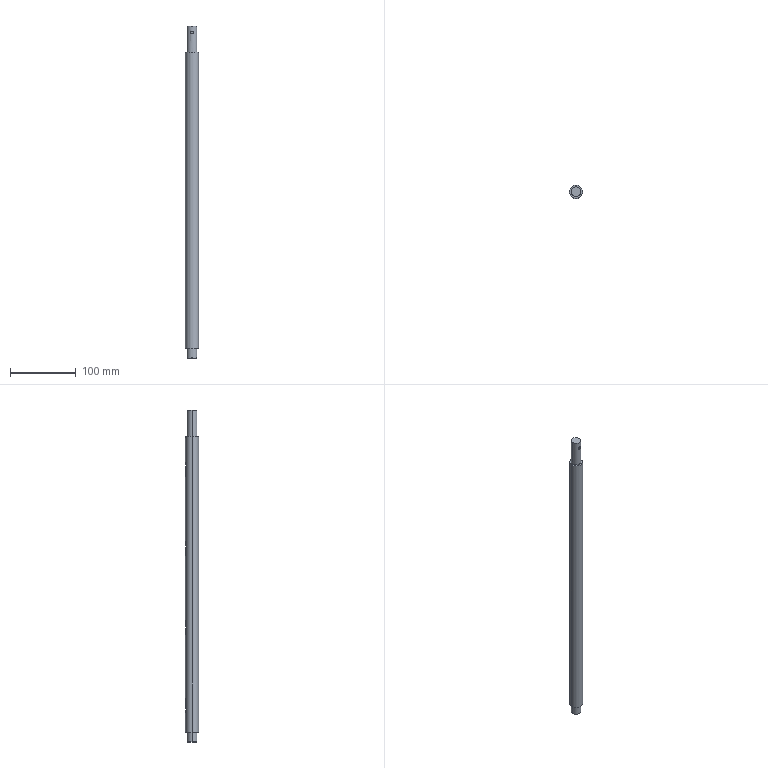Part | SolidWorks | features BaseBody 1 | 1 solid | 35 faces | box 20 x 20 x 505 mm | volume 149896 mm3 | plane 17 | cylinder 16 | cone 2 | commonest cylinder face diameters 6 x8 15 x4 4 x2 20 x2
STEP:
#1=CARTESIAN_POINT('',(2.,-6.,480.));
#2=VERTEX_POINT('',#1);
#3=CARTESIAN_POINT('',(-2.,-6.,480.));
#4=VERTEX_POINT('',#3);
#5=CARTESIAN_POINT('',(0.,-6.,480.));
#6=DIRECTION('',(0.,1.,0.));
#7=DIRECTION('',(1.,0.,0.));
#8=AXIS2_PLACEMENT_3D('',#5,#6,#7);
#9=CIRCLE('',#8,2.);
#10=EDGE_CURVE('',#2,#4,#9,.T.);
#11=ORIENTED_EDGE('',*,*,#10,.T.);
#12=CARTESIAN_POINT('',(-2.,-7.228,480.));
#13=VERTEX_POINT('',#12);
#14=CARTESIAN_POINT('',(-2.,-7.5,480.));
#15=DIRECTION('',(0.,-1.,0.));
#16=VECTOR('',#15,1000.);
#17=LINE('',#14,#16);
#18=EDGE_CURVE('',#4,#13,#17,.T.);
#19=ORIENTED_EDGE('',*,*,#18,.T.);
#20=CARTESIAN_POINT('',(2.,-7.228,480.));
#21=VERTEX_POINT('',#20);
#22=CARTESIAN_POINT('',(2.,-7.228,480.));
#23=CARTESIAN_POINT('',(2.,-7.228,479.867));
#24=CARTESIAN_POINT('',(1.987,-7.232,479.737));
#25=CARTESIAN_POINT('',(1.936,-7.246,479.481));
#26=CARTESIAN_POINT('',(1.897,-7.256,479.353));
#27=CARTESIAN_POINT('',(1.797,-7.282,479.112));
#28=CARTESIAN_POINT('',(1.735,-7.297,478.997));
#29=CARTESIAN_POINT('',(1.59,-7.33,478.78));
#30=CARTESIAN_POINT('',(1.506,-7.348,478.678));
#31=CARTESIAN_POINT('',(1.231,-7.401,478.403));
#32=CARTESIAN_POINT('',(1.009,-7.436,478.254));
#33=CARTESIAN_POINT('',(0.5289,-7.485,478.054));
#34=CARTESIAN_POINT('',(0.2655,-7.5,478.));
#35=CARTESIAN_POINT('',(-0.1326,-7.5,478.));
#36=CARTESIAN_POINT('',(-0.2629,-7.496,478.013));
#37=CARTESIAN_POINT('',(-0.5193,-7.483,478.064));
#38=CARTESIAN_POINT('',(-0.6466,-7.473,478.103));
#39=CARTESIAN_POINT('',(-0.8884,-7.448,478.203));
#40=CARTESIAN_POINT('',(-1.003,-7.433,478.265));
#41=CARTESIAN_POINT('',(-1.22,-7.401,478.41));
#42=CARTESIAN_POINT('',(-1.322,-7.383,478.494));
#43=CARTESIAN_POINT('',(-1.597,-7.33,478.769));
#44=CARTESIAN_POINT('',(-1.746,-7.295,478.991));
#45=CARTESIAN_POINT('',(-1.946,-7.244,479.471));
#46=CARTESIAN_POINT('',(-2.,-7.228,479.735));
#47=CARTESIAN_POINT('',(-2.,-7.228,480.));
#48=B_SPLINE_CURVE_WITH_KNOTS('',3,(#22,#23,#24,#25,#26,#27,#28,#29,#30,#31,#32,#33,#34,#35,#36,#37,#38,#39,#40,#41,#42,#43,#44,#45,#46,#47),.UNSPECIFIED.,.F.,.F.,(4,2,2,2,2,2,2,2,2,2,2,2,4),(0.009416,0.009808,0.0102,0.01059,0.01099,0.01177,0.01255,0.01295,0.01334,0.01373,0.01412,0.01491,0.01569),.UNSPECIFIED.);
#49=EDGE_CURVE('',#21,#13,#48,.T.);
#50=ORIENTED_EDGE('',*,*,#49,.F.);
#51=CARTESIAN_POINT('',(2.,-7.5,480.));
#52=DIRECTION('',(0.,-1.,0.));
#53=VECTOR('',#52,1000.);
#54=LINE('',#51,#53);
#55=EDGE_CURVE('',#2,#21,#54,.T.);
#56=ORIENTED_EDGE('',*,*,#55,.F.);
#57=EDGE_LOOP('',(#11,#19,#50,#56));
#58=FACE_OUTER_BOUND('',#57,.T.);
#59=CARTESIAN_POINT('',(0.,-7.5,480.));
#60=DIRECTION('',(0.,-1.,0.));
#61=DIRECTION('',(1.,0.,0.));
#62=AXIS2_PLACEMENT_3D('',#59,#60,#61);
#63=CYLINDRICAL_SURFACE('',#62,2.);
#64=ADVANCED_FACE('',(#58),#63,.F.);
#65=CARTESIAN_POINT('',(7.,0.,-15.));
#66=VERTEX_POINT('',#65);
#67=CARTESIAN_POINT('',(-7.,0.,-15.));
#68=VERTEX_POINT('',#67);
#69=CARTESIAN_POINT('',(0.,0.,-15.));
#70=DIRECTION('',(0.,0.,1.));
#71=DIRECTION('',(1.,0.,0.));
#72=AXIS2_PLACEMENT_3D('',#69,#70,#71);
#73=CIRCLE('',#72,7.);
#74=EDGE_CURVE('',#66,#68,#73,.T.);
#75=ORIENTED_EDGE('',*,*,#74,.T.);
#76=CARTESIAN_POINT('',(-7.5,0.,-14.5));
#77=VERTEX_POINT('',#76);
#78=CARTESIAN_POINT('',(-7.25,0.,-14.75));
#79=DIRECTION('',(-0.7071,0.,0.7071));
#80=VECTOR('',#79,1000.);
#81=LINE('',#78,#80);
#82=EDGE_CURVE('',#68,#77,#81,.T.);
#83=ORIENTED_EDGE('',*,*,#82,.T.);
#84=CARTESIAN_POINT('',(7.5,0.,-14.5));
#85=VERTEX_POINT('',#84);
#86=CARTESIAN_POINT('',(0.,0.,-14.5));
#87=DIRECTION('',(0.,0.,-1.));
#88=DIRECTION('',(1.,0.,0.));
#89=AXIS2_PLACEMENT_3D('',#86,#87,#88);
#90=CIRCLE('',#89,7.5);
#91=EDGE_CURVE('',#77,#85,#90,.T.);
#92=ORIENTED_EDGE('',*,*,#91,.T.);
#93=CARTESIAN_POINT('',(7.25,0.,-14.75));
#94=DIRECTION('',(0.7071,0.,0.7071));
#95=VECTOR('',#94,1000.);
#96=LINE('',#93,#95);
#97=EDGE_CURVE('',#66,#85,#96,.T.);
#98=ORIENTED_EDGE('',*,*,#97,.F.);
#99=EDGE_LOOP('',(#75,#83,#92,#98));
#100=FACE_OUTER_BOUND('',#99,.T.);
#101=CARTESIAN_POINT('',(0.,0.,-14.75));
#102=DIRECTION('',(0.,0.,1.));
#103=DIRECTION('',(1.,0.,0.));
#104=AXIS2_PLACEMENT_3D('',#101,#102,#103);
#105=CONICAL_SURFACE('',#104,7.25,0.7854);
#106=ADVANCED_FACE('',(#100),#105,.T.);
#107=ORIENTED_EDGE('',*,*,#91,.F.);
#108=CARTESIAN_POINT('',(-7.5,0.,0.));
#109=VERTEX_POINT('',#108);
#110=CARTESIAN_POINT('',(-7.5,0.,0.));
#111=DIRECTION('',(0.,0.,1.));
#112=VECTOR('',#111,1000.);
#113=LINE('',#110,#112);
#114=EDGE_CURVE('',#77,#109,#113,.T.);
#115=ORIENTED_EDGE('',*,*,#114,.T.);
#116=CARTESIAN_POINT('',(7.5,0.,0.));
#117=VERTEX_POINT('',#116);
#118=CARTESIAN_POINT('',(0.,0.,0.));
#119=DIRECTION('',(0.,0.,1.));
#120=DIRECTION('',(1.,0.,0.));
#121=AXIS2_PLACEMENT_3D('',#118,#119,#120);
#122=CIRCLE('',#121,7.5);
#123=EDGE_CURVE('',#117,#109,#122,.T.);
#124=ORIENTED_EDGE('',*,*,#123,.F.);
#125=CARTESIAN_POINT('',(7.5,0.,0.));
#126=DIRECTION('',(0.,0.,1.));
#127=VECTOR('',#126,1000.);
#128=LINE('',#125,#127);
#129=EDGE_CURVE('',#85,#117,#128,.T.);
#130=ORIENTED_EDGE('',*,*,#129,.F.);
#131=EDGE_LOOP('',(#107,#115,#124,#130));
#132=FACE_OUTER_BOUND('',#131,.T.);
#133=CARTESIAN_POINT('',(0.,0.,0.));
#134=DIRECTION('',(0.,0.,1.));
#135=DIRECTION('',(1.,0.,0.));
#136=AXIS2_PLACEMENT_3D('',#133,#134,#135);
#137=CYLINDRICAL_SURFACE('',#136,7.5);
#138=ADVANCED_FACE('',(#132),#137,.T.);
#139=CARTESIAN_POINT('',(7.5,0.,490.));
#140=VERTEX_POINT('',#139);
#141=CARTESIAN_POINT('',(-7.5,0.,490.));
#142=VERTEX_POINT('',#141);
#143=CARTESIAN_POINT('',(0.,0.,490.));
#144=DIRECTION('',(0.,0.,1.));
#145=DIRECTION('',(-1.,0.,0.));
#146=AXIS2_PLACEMENT_3D('',#143,#144,#145);
#147=CIRCLE('',#146,7.5);
#148=EDGE_CURVE('',#140,#142,#147,.T.);
#149=ORIENTED_EDGE('',*,*,#148,.F.);
#150=CARTESIAN_POINT('',(7.5,0.,450.));
#151=VERTEX_POINT('',#150);
#152=CARTESIAN_POINT('',(7.5,0.,450.));
#153=DIRECTION('',(0.,0.,-1.));
#154=VECTOR('',#153,1000.);
#155=LINE('',#152,#154);
#156=EDGE_CURVE('',#140,#151,#155,.T.);
#157=ORIENTED_EDGE('',*,*,#156,.T.);
#158=CARTESIAN_POINT('',(-7.5,0.,450.));
#159=VERTEX_POINT('',#158);
#160=CARTESIAN_POINT('',(0.,0.,450.));
#161=DIRECTION('',(0.,0.,-1.));
#162=DIRECTION('',(-1.,0.,0.));
#163=AXIS2_PLACEMENT_3D('',#160,#161,#162);
#164=CIRCLE('',#163,7.5);
#165=EDGE_CURVE('',#159,#151,#164,.T.);
#166=ORIENTED_EDGE('',*,*,#165,.F.);
#167=CARTESIAN_POINT('',(-7.5,0.,450.));
#168=DIRECTION('',(0.,0.,-1.));
#169=VECTOR('',#168,1000.);
#170=LINE('',#167,#169);
#171=EDGE_CURVE('',#142,#159,#170,.T.);
#172=ORIENTED_EDGE('',*,*,#171,.F.);
#173=EDGE_LOOP('',(#149,#157,#166,#172));
#174=FACE_OUTER_BOUND('',#173,.T.);
#175=CARTESIAN_POINT('',(0.,0.,450.));
#176=DIRECTION('',(0.,0.,-1.));
#177=DIRECTION('',(-1.,0.,0.));
#178=AXIS2_PLACEMENT_3D('',#175,#176,#177);
#179=CYLINDRICAL_SURFACE('',#178,7.5);
#180=ADVANCED_FACE('',(#174),#179,.T.);
#181=CARTESIAN_POINT('',(-3.,9.539,48.));
#182=VERTEX_POINT('',#181);
#183=CARTESIAN_POINT('',(-3.,9.539,32.));
#184=VERTEX_POINT('',#183);
#185=CARTESIAN_POINT('',(-3.,9.539,0.));
#186=DIRECTION('',(0.,0.,-1.));
#187=VECTOR('',#186,1000.);
#188=LINE('',#185,#187);
#189=EDGE_CURVE('',#182,#184,#188,.T.);
#190=ORIENTED_EDGE('',*,*,#189,.T.);
#191=CARTESIAN_POINT('',(3.,9.539,32.));
#192=VERTEX_POINT('',#191);
#193=CARTESIAN_POINT('',(-3.,9.539,32.));
#194=CARTESIAN_POINT('',(-3.,9.539,31.801));
#195=CARTESIAN_POINT('',(-2.98,9.546,31.605));
#196=CARTESIAN_POINT('',(-2.904,9.569,31.22));
#197=CARTESIAN_POINT('',(-2.845,9.587,31.029));
#198=CARTESIAN_POINT('',(-2.695,9.63,30.667));
#199=CARTESIAN_POINT('',(-2.602,9.656,30.495));
#200=CARTESIAN_POINT('',(-2.385,9.712,30.17));
#201=CARTESIAN_POINT('',(-2.259,9.742,30.017));
#202=CARTESIAN_POINT('',(-1.847,9.832,29.604));
#203=CARTESIAN_POINT('',(-1.515,9.891,29.381));
#204=CARTESIAN_POINT('',(-0.9743,9.954,29.156));
#205=CARTESIAN_POINT('',(-0.7844,9.971,29.098));
#206=CARTESIAN_POINT('',(-0.396,9.994,29.02));
#207=CARTESIAN_POINT('',(-0.1993,10.,29.));
#208=CARTESIAN_POINT('',(0.1994,10.,29.));
#209=CARTESIAN_POINT('',(0.3951,9.994,29.02));
#210=CARTESIAN_POINT('',(0.7799,9.971,29.097));
#211=CARTESIAN_POINT('',(0.971,9.954,29.155));
#212=CARTESIAN_POINT('',(1.334,9.912,29.306));
#213=CARTESIAN_POINT('',(1.505,9.887,29.398));
#214=CARTESIAN_POINT('',(1.831,9.832,29.615));
#215=CARTESIAN_POINT('',(1.984,9.802,29.741));
#216=CARTESIAN_POINT('',(2.396,9.713,30.153));
#217=CARTESIAN_POINT('',(2.619,9.652,30.486));
#218=CARTESIAN_POINT('',(2.844,9.587,31.026));
#219=CARTESIAN_POINT('',(2.902,9.57,31.216));
#220=CARTESIAN_POINT('',(2.98,9.546,31.604));
#221=CARTESIAN_POINT('',(3.,9.539,31.801));
#222=CARTESIAN_POINT('',(3.,9.539,32.));
#223=B_SPLINE_CURVE_WITH_KNOTS('',3,(#193,#194,#195,#196,#197,#198,#199,#200,#201,#202,#203,#204,#205,#206,#207,#208,#209,#210,#211,#212,#213,#214,#215,#216,#217,#218,#219,#220,#221,#222),.UNSPECIFIED.,.F.,.F.,(4,2,2,2,2,2,2,2,2,2,2,2,2,2,4),(0.,0.0005892,0.001178,0.001768,0.002357,0.003535,0.004125,0.004714,0.005303,0.005892,0.006482,0.007071,0.008249,0.008838,0.009428),.UNSPECIFIED.);
#224=EDGE_CURVE('',#184,#192,#223,.T.);
#225=ORIENTED_EDGE('',*,*,#224,.T.);
#226=CARTESIAN_POINT('',(3.,9.539,48.));
#227=VERTEX_POINT('',#226);
#228=CARTESIAN_POINT('',(3.,9.539,0.));
#229=DIRECTION('',(0.,0.,1.));
#230=VECTOR('',#229,1000.);
#231=LINE('',#228,#230);
#232=EDGE_CURVE('',#192,#227,#231,.T.);
#233=ORIENTED_EDGE('',*,*,#232,.T.);
#234=CARTESIAN_POINT('',(3.,9.539,48.));
#235=CARTESIAN_POINT('',(3.,9.539,48.199));
#236=CARTESIAN_POINT('',(2.98,9.546,48.395));
#237=CARTESIAN_POINT('',(2.904,9.569,48.78));
#238=CARTESIAN_POINT('',(2.845,9.587,48.971));
#239=CARTESIAN_POINT('',(2.695,9.63,49.333));
#240=CARTESIAN_POINT('',(2.602,9.656,49.505));
#241=CARTESIAN_POINT('',(2.385,9.712,49.83));
#242=CARTESIAN_POINT('',(2.259,9.742,49.983));
#243=CARTESIAN_POINT('',(1.847,9.832,50.396));
#244=CARTESIAN_POINT('',(1.515,9.891,50.619));
#245=CARTESIAN_POINT('',(0.9743,9.954,50.844));
#246=CARTESIAN_POINT('',(0.7844,9.971,50.902));
#247=CARTESIAN_POINT('',(0.396,9.994,50.98));
#248=CARTESIAN_POINT('',(0.1993,10.,51.));
#249=CARTESIAN_POINT('',(-0.1994,10.,51.));
#250=CARTESIAN_POINT('',(-0.3951,9.994,50.98));
#251=CARTESIAN_POINT('',(-0.7799,9.971,50.903));
#252=CARTESIAN_POINT('',(-0.971,9.954,50.845));
#253=CARTESIAN_POINT('',(-1.334,9.912,50.694));
#254=CARTESIAN_POINT('',(-1.505,9.887,50.602));
#255=CARTESIAN_POINT('',(-1.831,9.832,50.385));
#256=CARTESIAN_POINT('',(-1.984,9.802,50.259));
#257=CARTESIAN_POINT('',(-2.396,9.713,49.847));
#258=CARTESIAN_POINT('',(-2.619,9.652,49.514));
#259=CARTESIAN_POINT('',(-2.844,9.587,48.974));
#260=CARTESIAN_POINT('',(-2.902,9.57,48.784));
#261=CARTESIAN_POINT('',(-2.98,9.546,48.396));
#262=CARTESIAN_POINT('',(-3.,9.539,48.199));
#263=CARTESIAN_POINT('',(-3.,9.539,48.));
#264=B_SPLINE_CURVE_WITH_KNOTS('',3,(#234,#235,#236,#237,#238,#239,#240,#241,#242,#243,#244,#245,#246,#247,#248,#249,#250,#251,#252,#253,#254,#255,#256,#257,#258,#259,#260,#261,#262,#263),.UNSPECIFIED.,.F.,.F.,(4,2,2,2,2,2,2,2,2,2,2,2,2,2,4),(0.,0.0005892,0.001178,0.001768,0.002357,0.003535,0.004125,0.004714,0.005303,0.005892,0.006482,0.007071,0.008249,0.008838,0.009428),.UNSPECIFIED.);
#265=EDGE_CURVE('',#227,#182,#264,.T.);
#266=ORIENTED_EDGE('',*,*,#265,.T.);
#267=EDGE_LOOP('',(#190,#225,#233,#266));
#268=FACE_BOUND('',#267,.T.);
#269=CARTESIAN_POINT('',(-3.,9.539,168.));
#270=VERTEX_POINT('',#269);
#271=CARTESIAN_POINT('',(-3.,9.539,152.));
#272=VERTEX_POINT('',#271);
#273=CARTESIAN_POINT('',(-3.,9.539,0.));
#274=DIRECTION('',(0.,0.,-1.));
#275=VECTOR('',#274,1000.);
#276=LINE('',#273,#275);
#277=EDGE_CURVE('',#270,#272,#276,.T.);
#278=ORIENTED_EDGE('',*,*,#277,.T.);
#279=CARTESIAN_POINT('',(3.,9.539,152.));
#280=VERTEX_POINT('',#279);
#281=CARTESIAN_POINT('',(-3.,9.539,152.));
#282=CARTESIAN_POINT('',(-3.,9.539,151.801));
#283=CARTESIAN_POINT('',(-2.98,9.546,151.605));
#284=CARTESIAN_POINT('',(-2.904,9.569,151.22));
#285=CARTESIAN_POINT('',(-2.845,9.587,151.029));
#286=CARTESIAN_POINT('',(-2.695,9.63,150.667));
#287=CARTESIAN_POINT('',(-2.602,9.656,150.495));
#288=CARTESIAN_POINT('',(-2.385,9.712,150.17));
#289=CARTESIAN_POINT('',(-2.259,9.742,150.017));
#290=CARTESIAN_POINT('',(-1.847,9.832,149.604));
#291=CARTESIAN_POINT('',(-1.515,9.891,149.381));
#292=CARTESIAN_POINT('',(-0.9743,9.954,149.156));
#293=CARTESIAN_POINT('',(-0.7844,9.971,149.098));
#294=CARTESIAN_POINT('',(-0.396,9.994,149.02));
#295=CARTESIAN_POINT('',(-0.1993,10.,149.));
#296=CARTESIAN_POINT('',(0.1994,10.,149.));
#297=CARTESIAN_POINT('',(0.3951,9.994,149.02));
#298=CARTESIAN_POINT('',(0.7799,9.971,149.097));
#299=CARTESIAN_POINT('',(0.971,9.954,149.155));
#300=CARTESIAN_POINT('',(1.334,9.912,149.306));
#301=CARTESIAN_POINT('',(1.505,9.887,149.398));
#302=CARTESIAN_POINT('',(1.831,9.832,149.615));
#303=CARTESIAN_POINT('',(1.984,9.802,149.741));
#304=CARTESIAN_POINT('',(2.396,9.713,150.153));
#305=CARTESIAN_POINT('',(2.619,9.652,150.486));
#306=CARTESIAN_POINT('',(2.844,9.587,151.026));
#307=CARTESIAN_POINT('',(2.902,9.57,151.216));
#308=CARTESIAN_POINT('',(2.98,9.546,151.604));
#309=CARTESIAN_POINT('',(3.,9.539,151.801));
#310=CARTESIAN_POINT('',(3.,9.539,152.));
#311=B_SPLINE_CURVE_WITH_KNOTS('',3,(#281,#282,#283,#284,#285,#286,#287,#288,#289,#290,#291,#292,#293,#294,#295,#296,#297,#298,#299,#300,#301,#302,#303,#304,#305,#306,#307,#308,#309,#310),.UNSPECIFIED.,.F.,.F.,(4,2,2,2,2,2,2,2,2,2,2,2,2,2,4),(0.,0.0005892,0.001178,0.001768,0.002357,0.003535,0.004125,0.004714,0.005303,0.005892,0.006482,0.007071,0.008249,0.008838,0.009428),.UNSPECIFIED.);
#312=EDGE_CURVE('',#272,#280,#311,.T.);
#313=ORIENTED_EDGE('',*,*,#312,.T.);
#314=CARTESIAN_POINT('',(3.,9.539,168.));
#315=VERTEX_POINT('',#314);
#316=CARTESIAN_POINT('',(3.,9.539,0.));
#317=DIRECTION('',(0.,0.,1.));
#318=VECTOR('',#317,1000.);
#319=LINE('',#316,#318);
#320=EDGE_CURVE('',#280,#315,#319,.T.);
#321=ORIENTED_EDGE('',*,*,#320,.T.);
#322=CARTESIAN_POINT('',(3.,9.539,168.));
#323=CARTESIAN_POINT('',(3.,9.539,168.199));
#324=CARTESIAN_POINT('',(2.98,9.546,168.395));
#325=CARTESIAN_POINT('',(2.904,9.569,168.78));
#326=CARTESIAN_POINT('',(2.845,9.587,168.971));
#327=CARTESIAN_POINT('',(2.695,9.63,169.333));
#328=CARTESIAN_POINT('',(2.602,9.656,169.505));
#329=CARTESIAN_POINT('',(2.385,9.712,169.83));
#330=CARTESIAN_POINT('',(2.259,9.742,169.983));
#331=CARTESIAN_POINT('',(1.847,9.832,170.396));
#332=CARTESIAN_POINT('',(1.515,9.891,170.619));
#333=CARTESIAN_POINT('',(0.9743,9.954,170.844));
#334=CARTESIAN_POINT('',(0.7844,9.971,170.902));
#335=CARTESIAN_POINT('',(0.396,9.994,170.98));
#336=CARTESIAN_POINT('',(0.1993,10.,171.));
#337=CARTESIAN_POINT('',(-0.1994,10.,171.));
#338=CARTESIAN_POINT('',(-0.3951,9.994,170.98));
#339=CARTESIAN_POINT('',(-0.7799,9.971,170.903));
#340=CARTESIAN_POINT('',(-0.971,9.954,170.845));
#341=CARTESIAN_POINT('',(-1.334,9.912,170.694));
#342=CARTESIAN_POINT('',(-1.505,9.887,170.602));
#343=CARTESIAN_POINT('',(-1.831,9.832,170.385));
#344=CARTESIAN_POINT('',(-1.984,9.802,170.259));
#345=CARTESIAN_POINT('',(-2.396,9.713,169.847));
#346=CARTESIAN_POINT('',(-2.619,9.652,169.514));
#347=CARTESIAN_POINT('',(-2.844,9.587,168.974));
#348=CARTESIAN_POINT('',(-2.902,9.57,168.784));
#349=CARTESIAN_POINT('',(-2.98,9.546,168.396));
#350=CARTESIAN_POINT('',(-3.,9.539,168.199));
#351=CARTESIAN_POINT('',(-3.,9.539,168.));
#352=B_SPLINE_CURVE_WITH_KNOTS('',3,(#322,#323,#324,#325,#326,#327,#328,#329,#330,#331,#332,#333,#334,#335,#336,#337,#338,#339,#340,#341,#342,#343,#344,#345,#346,#347,#348,#349,#350,#351),.UNSPECIFIED.,.F.,.F.,(4,2,2,2,2,2,2,2,2,2,2,2,2,2,4),(0.,0.0005892,0.001178,0.001768,0.002357,0.003535,0.004125,0.004714,0.005303,0.005892,0.006482,0.007071,0.008249,0.008838,0.009428),.UNSPECIFIED.);
#353=EDGE_CURVE('',#315,#270,#352,.T.);
#354=ORIENTED_EDGE('',*,*,#353,.T.);
#355=EDGE_LOOP('',(#278,#313,#321,#354));
#356=FACE_BOUND('',#355,.T.);
#357=CARTESIAN_POINT('',(-3.,9.539,288.));
#358=VERTEX_POINT('',#357);
#359=CARTESIAN_POINT('',(-3.,9.539,272.));
#360=VERTEX_POINT('',#359);
#361=CARTESIAN_POINT('',(-3.,9.539,0.));
#362=DIRECTION('',(0.,0.,-1.));
#363=VECTOR('',#362,1000.);
#364=LINE('',#361,#363);
#365=EDGE_CURVE('',#358,#360,#364,.T.);
#366=ORIENTED_EDGE('',*,*,#365,.T.);
#367=CARTESIAN_POINT('',(3.,9.539,272.));
#368=VERTEX_POINT('',#367);
#369=CARTESIAN_POINT('',(-3.,9.539,272.));
#370=CARTESIAN_POINT('',(-3.,9.539,271.801));
#371=CARTESIAN_POINT('',(-2.98,9.546,271.605));
#372=CARTESIAN_POINT('',(-2.904,9.569,271.22));
#373=CARTESIAN_POINT('',(-2.845,9.587,271.029));
#374=CARTESIAN_POINT('',(-2.695,9.63,270.667));
#375=CARTESIAN_POINT('',(-2.602,9.656,270.495));
#376=CARTESIAN_POINT('',(-2.385,9.712,270.17));
#377=CARTESIAN_POINT('',(-2.259,9.742,270.017));
#378=CARTESIAN_POINT('',(-1.847,9.832,269.604));
#379=CARTESIAN_POINT('',(-1.515,9.891,269.381));
#380=CARTESIAN_POINT('',(-0.9743,9.954,269.156));
#381=CARTESIAN_POINT('',(-0.7844,9.971,269.098));
#382=CARTESIAN_POINT('',(-0.396,9.994,269.02));
#383=CARTESIAN_POINT('',(-0.1993,10.,269.));
#384=CARTESIAN_POINT('',(0.1994,10.,269.));
#385=CARTESIAN_POINT('',(0.3951,9.994,269.02));
#386=CARTESIAN_POINT('',(0.7799,9.971,269.097));
#387=CARTESIAN_POINT('',(0.971,9.954,269.155));
#388=CARTESIAN_POINT('',(1.334,9.912,269.306));
#389=CARTESIAN_POINT('',(1.505,9.887,269.398));
#390=CARTESIAN_POINT('',(1.831,9.832,269.615));
#391=CARTESIAN_POINT('',(1.984,9.802,269.741));
#392=CARTESIAN_POINT('',(2.396,9.713,270.153));
#393=CARTESIAN_POINT('',(2.619,9.652,270.486));
#394=CARTESIAN_POINT('',(2.844,9.587,271.026));
#395=CARTESIAN_POINT('',(2.902,9.57,271.216));
#396=CARTESIAN_POINT('',(2.98,9.546,271.604));
#397=CARTESIAN_POINT('',(3.,9.539,271.801));
#398=CARTESIAN_POINT('',(3.,9.539,272.));
#399=B_SPLINE_CURVE_WITH_KNOTS('',3,(#369,#370,#371,#372,#373,#374,#375,#376,#377,#378,#379,#380,#381,#382,#383,#384,#385,#386,#387,#388,#389,#390,#391,#392,#393,#394,#395,#396,#397,#398),.UNSPECIFIED.,.F.,.F.,(4,2,2,2,2,2,2,2,2,2,2,2,2,2,4),(0.,0.0005892,0.001178,0.001768,0.002357,0.003535,0.004125,0.004714,0.005303,0.005892,0.006482,0.007071,0.008249,0.008838,0.009428),.UNSPECIFIED.);
#400=EDGE_CURVE('',#360,#368,#399,.T.);
#401=ORIENTED_EDGE('',*,*,#400,.T.);
#402=CARTESIAN_POINT('',(3.,9.539,288.));
#403=VERTEX_POINT('',#402);
#404=CARTESIAN_POINT('',(3.,9.539,0.));
#405=DIRECTION('',(0.,0.,1.));
#406=VECTOR('',#405,1000.);
#407=LINE('',#404,#406);
#408=EDGE_CURVE('',#368,#403,#407,.T.);
#409=ORIENTED_EDGE('',*,*,#408,.T.);
#410=CARTESIAN_POINT('',(3.,9.539,288.));
#411=CARTESIAN_POINT('',(3.,9.539,288.199));
#412=CARTESIAN_POINT('',(2.98,9.546,288.395));
#413=CARTESIAN_POINT('',(2.904,9.569,288.78));
#414=CARTESIAN_POINT('',(2.845,9.587,288.971));
#415=CARTESIAN_POINT('',(2.695,9.63,289.333));
#416=CARTESIAN_POINT('',(2.602,9.656,289.505));
#417=CARTESIAN_POINT('',(2.385,9.712,289.83));
#418=CARTESIAN_POINT('',(2.259,9.742,289.983));
#419=CARTESIAN_POINT('',(1.847,9.832,290.396));
#420=CARTESIAN_POINT('',(1.515,9.891,290.619));
#421=CARTESIAN_POINT('',(0.9743,9.954,290.844));
#422=CARTESIAN_POINT('',(0.7844,9.971,290.902));
#423=CARTESIAN_POINT('',(0.396,9.994,290.98));
#424=CARTESIAN_POINT('',(0.1993,10.,291.));
#425=CARTESIAN_POINT('',(-0.1994,10.,291.));
#426=CARTESIAN_POINT('',(-0.3951,9.994,290.98));
#427=CARTESIAN_POINT('',(-0.7799,9.971,290.903));
#428=CARTESIAN_POINT('',(-0.971,9.954,290.845));
#429=CARTESIAN_POINT('',(-1.334,9.912,290.694));
#430=CARTESIAN_POINT('',(-1.505,9.887,290.602));
#431=CARTESIAN_POINT('',(-1.831,9.832,290.385));
#432=CARTESIAN_POINT('',(-1.984,9.802,290.259));
#433=CARTESIAN_POINT('',(-2.396,9.713,289.847));
#434=CARTESIAN_POINT('',(-2.619,9.652,289.514));
#435=CARTESIAN_POINT('',(-2.844,9.587,288.974));
#436=CARTESIAN_POINT('',(-2.902,9.57,288.784));
#437=CARTESIAN_POINT('',(-2.98,9.546,288.396));
#438=CARTESIAN_POINT('',(-3.,9.539,288.199));
#439=CARTESIAN_POINT('',(-3.,9.539,288.));
#440=B_SPLINE_CURVE_WITH_KNOTS('',3,(#410,#411,#412,#413,#414,#415,#416,#417,#418,#419,#420,#421,#422,#423,#424,#425,#426,#427,#428,#429,#430,#431,#432,#433,#434,#435,#436,#437,#438,#439),.UNSPECIFIED.,.F.,.F.,(4,2,2,2,2,2,2,2,2,2,2,2,2,2,4),(0.,0.0005892,0.001178,0.001768,0.002357,0.003535,0.004125,0.004714,0.005303,0.005892,0.006482,0.007071,0.008249,0.008838,0.009428),.UNSPECIFIED.);
#441=EDGE_CURVE('',#403,#358,#440,.T.);
#442=ORIENTED_EDGE('',*,*,#441,.T.);
#443=EDGE_LOOP('',(#366,#401,#409,#442));
#444=FACE_BOUND('',#443,.T.);
#445=CARTESIAN_POINT('',(-3.,9.539,408.));
#446=VERTEX_POINT('',#445);
#447=CARTESIAN_POINT('',(-3.,9.539,392.));
#448=VERTEX_POINT('',#447);
#449=CARTESIAN_POINT('',(-3.,9.539,0.));
#450=DIRECTION('',(0.,0.,-1.));
#451=VECTOR('',#450,1000.);
#452=LINE('',#449,#451);
#453=EDGE_CURVE('',#446,#448,#452,.T.);
#454=ORIENTED_EDGE('',*,*,#453,.T.);
#455=CARTESIAN_POINT('',(3.,9.539,392.));
#456=VERTEX_POINT('',#455);
#457=CARTESIAN_POINT('',(-3.,9.539,392.));
#458=CARTESIAN_POINT('',(-3.,9.539,391.801));
#459=CARTESIAN_POINT('',(-2.98,9.546,391.605));
#460=CARTESIAN_POINT('',(-2.904,9.569,391.22));
#461=CARTESIAN_POINT('',(-2.845,9.587,391.029));
#462=CARTESIAN_POINT('',(-2.695,9.63,390.667));
#463=CARTESIAN_POINT('',(-2.602,9.656,390.495));
#464=CARTESIAN_POINT('',(-2.385,9.712,390.17));
#465=CARTESIAN_POINT('',(-2.259,9.742,390.017));
#466=CARTESIAN_POINT('',(-1.847,9.832,389.604));
#467=CARTESIAN_POINT('',(-1.515,9.891,389.381));
#468=CARTESIAN_POINT('',(-0.9743,9.954,389.156));
#469=CARTESIAN_POINT('',(-0.7844,9.971,389.098));
#470=CARTESIAN_POINT('',(-0.396,9.994,389.02));
#471=CARTESIAN_POINT('',(-0.1993,10.,389.));
#472=CARTESIAN_POINT('',(0.1994,10.,389.));
#473=CARTESIAN_POINT('',(0.3951,9.994,389.02));
#474=CARTESIAN_POINT('',(0.7799,9.971,389.097));
#475=CARTESIAN_POINT('',(0.971,9.954,389.155));
#476=CARTESIAN_POINT('',(1.334,9.912,389.306));
#477=CARTESIAN_POINT('',(1.505,9.887,389.398));
#478=CARTESIAN_POINT('',(1.831,9.832,389.615));
#479=CARTESIAN_POINT('',(1.984,9.802,389.741));
#480=CARTESIAN_POINT('',(2.396,9.713,390.153));
#481=CARTESIAN_POINT('',(2.619,9.652,390.486));
#482=CARTESIAN_POINT('',(2.844,9.587,391.026));
#483=CARTESIAN_POINT('',(2.902,9.57,391.216));
#484=CARTESIAN_POINT('',(2.98,9.546,391.604));
#485=CARTESIAN_POINT('',(3.,9.539,391.801));
#486=CARTESIAN_POINT('',(3.,9.539,392.));
#487=B_SPLINE_CURVE_WITH_KNOTS('',3,(#457,#458,#459,#460,#461,#462,#463,#464,#465,#466,#467,#468,#469,#470,#471,#472,#473,#474,#475,#476,#477,#478,#479,#480,#481,#482,#483,#484,#485,#486),.UNSPECIFIED.,.F.,.F.,(4,2,2,2,2,2,2,2,2,2,2,2,2,2,4),(0.,0.0005892,0.001178,0.001768,0.002357,0.003535,0.004125,0.004714,0.005303,0.005892,0.006482,0.007071,0.008249,0.008838,0.009428),.UNSPECIFIED.);
#488=EDGE_CURVE('',#448,#456,#487,.T.);
#489=ORIENTED_EDGE('',*,*,#488,.T.);
#490=CARTESIAN_POINT('',(3.,9.539,408.));
#491=VERTEX_POINT('',#490);
#492=CARTESIAN_POINT('',(3.,9.539,0.));
#493=DIRECTION('',(0.,0.,1.));
#494=VECTOR('',#493,1000.);
#495=LINE('',#492,#494);
#496=EDGE_CURVE('',#456,#491,#495,.T.);
#497=ORIENTED_EDGE('',*,*,#496,.T.);
#498=CARTESIAN_POINT('',(3.,9.539,408.));
#499=CARTESIAN_POINT('',(3.,9.539,408.199));
#500=CARTESIAN_POINT('',(2.98,9.546,408.395));
#501=CARTESIAN_POINT('',(2.904,9.569,408.78));
#502=CARTESIAN_POINT('',(2.845,9.587,408.971));
#503=CARTESIAN_POINT('',(2.695,9.63,409.333));
#504=CARTESIAN_POINT('',(2.602,9.656,409.505));
#505=CARTESIAN_POINT('',(2.385,9.712,409.83));
#506=CARTESIAN_POINT('',(2.259,9.742,409.983));
#507=CARTESIAN_POINT('',(1.847,9.832,410.396));
#508=CARTESIAN_POINT('',(1.515,9.891,410.619));
#509=CARTESIAN_POINT('',(0.9743,9.954,410.844));
#510=CARTESIAN_POINT('',(0.7844,9.971,410.902));
#511=CARTESIAN_POINT('',(0.396,9.994,410.98));
#512=CARTESIAN_POINT('',(0.1993,10.,411.));
#513=CARTESIAN_POINT('',(-0.1994,10.,411.));
#514=CARTESIAN_POINT('',(-0.3951,9.994,410.98));
#515=CARTESIAN_POINT('',(-0.7799,9.971,410.903));
#516=CARTESIAN_POINT('',(-0.971,9.954,410.845));
#517=CARTESIAN_POINT('',(-1.334,9.912,410.694));
#518=CARTESIAN_POINT('',(-1.505,9.887,410.602));
#519=CARTESIAN_POINT('',(-1.831,9.832,410.385));
#520=CARTESIAN_POINT('',(-1.984,9.802,410.259));
#521=CARTESIAN_POINT('',(-2.396,9.713,409.847));
#522=CARTESIAN_POINT('',(-2.619,9.652,409.514));
#523=CARTESIAN_POINT('',(-2.844,9.587,408.974));
#524=CARTESIAN_POINT('',(-2.902,9.57,408.784));
#525=CARTESIAN_POINT('',(-2.98,9.546,408.396));
#526=CARTESIAN_POINT('',(-3.,9.539,408.199));
#527=CARTESIAN_POINT('',(-3.,9.539,408.));
#528=B_SPLINE_CURVE_WITH_KNOTS('',3,(#498,#499,#500,#501,#502,#503,#504,#505,#506,#507,#508,#509,#510,#511,#512,#513,#514,#515,#516,#517,#518,#519,#520,#521,#522,#523,#524,#525,#526,#527),.UNSPECIFIED.,.F.,.F.,(4,2,2,2,2,2,2,2,2,2,2,2,2,2,4),(0.,0.0005892,0.001178,0.001768,0.002357,0.003535,0.004125,0.004714,0.005303,0.005892,0.006482,0.007071,0.008249,0.008838,0.009428),.UNSPECIFIED.);
#529=EDGE_CURVE('',#491,#446,#528,.T.);
#530=ORIENTED_EDGE('',*,*,#529,.T.);
#531=EDGE_LOOP('',(#454,#489,#497,#530));
#532=FACE_BOUND('',#531,.T.);
#533=CARTESIAN_POINT('',(10.,0.,450.));
#534=VERTEX_POINT('',#533);
#535=CARTESIAN_POINT('',(-10.,0.,450.));
#536=VERTEX_POINT('',#535);
#537=CARTESIAN_POINT('',(0.,0.,450.));
#538=DIRECTION('',(0.,0.,1.));
#539=DIRECTION('',(-1.,0.,0.));
#540=AXIS2_PLACEMENT_3D('',#537,#538,#539);
#541=CIRCLE('',#540,10.);
#542=EDGE_CURVE('',#534,#536,#541,.T.);
#543=ORIENTED_EDGE('',*,*,#542,.F.);
#544=CARTESIAN_POINT('',(10.,0.,0.));
#545=VERTEX_POINT('',#544);
#546=CARTESIAN_POINT('',(10.,0.,0.));
#547=DIRECTION('',(0.,0.,-1.));
#548=VECTOR('',#547,1000.);
#549=LINE('',#546,#548);
#550=EDGE_CURVE('',#534,#545,#549,.T.);
#551=ORIENTED_EDGE('',*,*,#550,.T.);
#552=CARTESIAN_POINT('',(-10.,0.,0.));
#553=VERTEX_POINT('',#552);
#554=CARTESIAN_POINT('',(0.,0.,0.));
#555=DIRECTION('',(0.,0.,-1.));
#556=DIRECTION('',(-1.,0.,0.));
#557=AXIS2_PLACEMENT_3D('',#554,#555,#556);
#558=CIRCLE('',#557,10.);
#559=EDGE_CURVE('',#553,#545,#558,.T.);
#560=ORIENTED_EDGE('',*,*,#559,.F.);
#561=CARTESIAN_POINT('',(-10.,0.,0.));
#562=DIRECTION('',(0.,0.,-1.));
#563=VECTOR('',#562,1000.);
#564=LINE('',#561,#563);
#565=EDGE_CURVE('',#536,#553,#564,.T.);
#566=ORIENTED_EDGE('',*,*,#565,.F.);
#567=EDGE_LOOP('',(#543,#551,#560,#566));
#568=FACE_OUTER_BOUND('',#567,.T.);
#569=CARTESIAN_POINT('',(0.,0.,0.));
#570=DIRECTION('',(0.,0.,-1.));
#571=DIRECTION('',(-1.,0.,0.));
#572=AXIS2_PLACEMENT_3D('',#569,#570,#571);
#573=CYLINDRICAL_SURFACE('',#572,10.);
#574=ADVANCED_FACE('',(#268,#356,#444,#532,#568),#573,.T.);
#575=ORIENTED_EDGE('',*,*,#10,.F.);
#576=CARTESIAN_POINT('',(0.,-6.,480.));
#577=DIRECTION('',(0.,1.,0.));
#578=DIRECTION('',(1.,0.,0.));
#579=AXIS2_PLACEMENT_3D('',#576,#577,#578);
#580=CIRCLE('',#579,2.);
#581=EDGE_CURVE('',#4,#2,#580,.T.);
#582=ORIENTED_EDGE('',*,*,#581,.F.);
#583=EDGE_LOOP('',(#575,#582));
#584=FACE_OUTER_BOUND('',#583,.T.);
#585=CARTESIAN_POINT('',(0.,-6.,480.));
#586=DIRECTION('',(0.,1.,0.));
#587=DIRECTION('',(1.,0.,0.));
#588=AXIS2_PLACEMENT_3D('',#585,#586,#587);
#589=PLANE('',#588);
#590=ADVANCED_FACE('',(#584),#589,.F.);
#591=ORIENTED_EDGE('',*,*,#232,.F.);
#592=CARTESIAN_POINT('',(3.,7.5,32.));
#593=VERTEX_POINT('',#592);
#594=CARTESIAN_POINT('',(3.,10.,32.));
#595=DIRECTION('',(0.,-1.,0.));
#596=VECTOR('',#595,1000.);
#597=LINE('',#594,#596);
#598=EDGE_CURVE('',#192,#593,#597,.T.);
#599=ORIENTED_EDGE('',*,*,#598,.T.);
#600=CARTESIAN_POINT('',(3.,7.5,48.));
#601=VERTEX_POINT('',#600);
#602=CARTESIAN_POINT('',(3.,7.5,48.));
#603=DIRECTION('',(0.,0.,1.));
#604=VECTOR('',#603,1000.);
#605=LINE('',#602,#604);
#606=EDGE_CURVE('',#593,#601,#605,.T.);
#607=ORIENTED_EDGE('',*,*,#606,.T.);
#608=CARTESIAN_POINT('',(3.,10.,48.));
#609=DIRECTION('',(0.,-1.,0.));
#610=VECTOR('',#609,1000.);
#611=LINE('',#608,#610);
#612=EDGE_CURVE('',#227,#601,#611,.T.);
#613=ORIENTED_EDGE('',*,*,#612,.F.);
#614=EDGE_LOOP('',(#591,#599,#607,#613));
#615=FACE_OUTER_BOUND('',#614,.T.);
#616=CARTESIAN_POINT('',(3.,10.,32.));
#617=DIRECTION('',(1.,0.,0.));
#618=DIRECTION('',(0.,0.,1.));
#619=AXIS2_PLACEMENT_3D('',#616,#617,#618);
#620=PLANE('',#619);
#621=ADVANCED_FACE('',(#615),#620,.F.);
#622=ORIENTED_EDGE('',*,*,#265,.F.);
#623=ORIENTED_EDGE('',*,*,#612,.T.);
#624=CARTESIAN_POINT('',(-3.,7.5,48.));
#625=VERTEX_POINT('',#624);
#626=CARTESIAN_POINT('',(0.,7.5,48.));
#627=DIRECTION('',(0.,-1.,0.));
#628=DIRECTION('',(-1.,0.,0.));
#629=AXIS2_PLACEMENT_3D('',#626,#627,#628);
#630=CIRCLE('',#629,3.);
#631=EDGE_CURVE('',#601,#625,#630,.T.);
#632=ORIENTED_EDGE('',*,*,#631,.T.);
#633=CARTESIAN_POINT('',(-3.,10.,48.));
#634=DIRECTION('',(0.,-1.,0.));
#635=VECTOR('',#634,1000.);
#636=LINE('',#633,#635);
#637=EDGE_CURVE('',#182,#625,#636,.T.);
#638=ORIENTED_EDGE('',*,*,#637,.F.);
#639=EDGE_LOOP('',(#622,#623,#632,#638));
#640=FACE_OUTER_BOUND('',#639,.T.);
#641=CARTESIAN_POINT('',(0.,10.,48.));
#642=DIRECTION('',(0.,1.,0.));
#643=DIRECTION('',(-1.,0.,0.));
#644=AXIS2_PLACEMENT_3D('',#641,#642,#643);
#645=CYLINDRICAL_SURFACE('',#644,3.);
#646=ADVANCED_FACE('',(#640),#645,.F.);
#647=ORIENTED_EDGE('',*,*,#189,.F.);
#648=ORIENTED_EDGE('',*,*,#637,.T.);
#649=CARTESIAN_POINT('',(-3.,7.5,32.));
#650=VERTEX_POINT('',#649);
#651=CARTESIAN_POINT('',(-3.,7.5,32.));
#652=DIRECTION('',(0.,0.,-1.));
#653=VECTOR('',#652,1000.);
#654=LINE('',#651,#653);
#655=EDGE_CURVE('',#625,#650,#654,.T.);
#656=ORIENTED_EDGE('',*,*,#655,.T.);
#657=CARTESIAN_POINT('',(-3.,10.,32.));
#658=DIRECTION('',(0.,-1.,0.));
#659=VECTOR('',#658,1000.);
#660=LINE('',#657,#659);
#661=EDGE_CURVE('',#184,#650,#660,.T.);
#662=ORIENTED_EDGE('',*,*,#661,.F.);
#663=EDGE_LOOP('',(#647,#648,#656,#662));
#664=FACE_OUTER_BOUND('',#663,.T.);
#665=CARTESIAN_POINT('',(-3.,10.,48.));
#666=DIRECTION('',(-1.,0.,0.));
#667=DIRECTION('',(0.,0.,1.));
#668=AXIS2_PLACEMENT_3D('',#665,#666,#667);
#669=PLANE('',#668);
#670=ADVANCED_FACE('',(#664),#669,.F.);
#671=ORIENTED_EDGE('',*,*,#598,.F.);
#672=ORIENTED_EDGE('',*,*,#224,.F.);
#673=ORIENTED_EDGE('',*,*,#661,.T.);
#674=CARTESIAN_POINT('',(0.,7.5,32.));
#675=DIRECTION('',(0.,-1.,0.));
#676=DIRECTION('',(1.,0.,0.));
#677=AXIS2_PLACEMENT_3D('',#674,#675,#676);
#678=CIRCLE('',#677,3.);
#679=EDGE_CURVE('',#650,#593,#678,.T.);
#680=ORIENTED_EDGE('',*,*,#679,.T.);
#681=EDGE_LOOP('',(#671,#672,#673,#680));
#682=FACE_OUTER_BOUND('',#681,.T.);
#683=CARTESIAN_POINT('',(0.,10.,32.));
#684=DIRECTION('',(0.,1.,0.));
#685=DIRECTION('',(1.,0.,0.));
#686=AXIS2_PLACEMENT_3D('',#683,#684,#685);
#687=CYLINDRICAL_SURFACE('',#686,3.);
#688=ADVANCED_FACE('',(#682),#687,.F.);
#689=ORIENTED_EDGE('',*,*,#679,.F.);
#690=ORIENTED_EDGE('',*,*,#655,.F.);
#691=ORIENTED_EDGE('',*,*,#631,.F.);
#692=ORIENTED_EDGE('',*,*,#606,.F.);
#693=EDGE_LOOP('',(#689,#690,#691,#692));
#694=FACE_OUTER_BOUND('',#693,.T.);
#695=CARTESIAN_POINT('',(0.,7.5,30.967));
#696=DIRECTION('',(0.,1.,0.));
#697=DIRECTION('',(1.,0.,0.));
#698=AXIS2_PLACEMENT_3D('',#695,#696,#697);
#699=PLANE('',#698);
#700=ADVANCED_FACE('',(#694),#699,.T.);
#701=ORIENTED_EDGE('',*,*,#320,.F.);
#702=CARTESIAN_POINT('',(3.,7.5,152.));
#703=VERTEX_POINT('',#702);
#704=CARTESIAN_POINT('',(3.,10.,152.));
#705=DIRECTION('',(0.,-1.,0.));
#706=VECTOR('',#705,1000.);
#707=LINE('',#704,#706);
#708=EDGE_CURVE('',#280,#703,#707,.T.);
#709=ORIENTED_EDGE('',*,*,#708,.T.);
#710=CARTESIAN_POINT('',(3.,7.5,168.));
#711=VERTEX_POINT('',#710);
#712=CARTESIAN_POINT('',(3.,7.5,168.));
#713=DIRECTION('',(0.,0.,1.));
#714=VECTOR('',#713,1000.);
#715=LINE('',#712,#714);
#716=EDGE_CURVE('',#703,#711,#715,.T.);
#717=ORIENTED_EDGE('',*,*,#716,.T.);
#718=CARTESIAN_POINT('',(3.,10.,168.));
#719=DIRECTION('',(0.,-1.,0.));
#720=VECTOR('',#719,1000.);
#721=LINE('',#718,#720);
#722=EDGE_CURVE('',#315,#711,#721,.T.);
#723=ORIENTED_EDGE('',*,*,#722,.F.);
#724=EDGE_LOOP('',(#701,#709,#717,#723));
#725=FACE_OUTER_BOUND('',#724,.T.);
#726=CARTESIAN_POINT('',(3.,10.,152.));
#727=DIRECTION('',(1.,0.,0.));
#728=DIRECTION('',(0.,0.,1.));
#729=AXIS2_PLACEMENT_3D('',#726,#727,#728);
#730=PLANE('',#729);
#731=ADVANCED_FACE('',(#725),#730,.F.);
#732=ORIENTED_EDGE('',*,*,#353,.F.);
#733=ORIENTED_EDGE('',*,*,#722,.T.);
#734=CARTESIAN_POINT('',(-3.,7.5,168.));
#735=VERTEX_POINT('',#734);
#736=CARTESIAN_POINT('',(0.,7.5,168.));
#737=DIRECTION('',(0.,-1.,0.));
#738=DIRECTION('',(-1.,0.,0.));
#739=AXIS2_PLACEMENT_3D('',#736,#737,#738);
#740=CIRCLE('',#739,3.);
#741=EDGE_CURVE('',#711,#735,#740,.T.);
#742=ORIENTED_EDGE('',*,*,#741,.T.);
#743=CARTESIAN_POINT('',(-3.,10.,168.));
#744=DIRECTION('',(0.,-1.,0.));
#745=VECTOR('',#744,1000.);
#746=LINE('',#743,#745);
#747=EDGE_CURVE('',#270,#735,#746,.T.);
#748=ORIENTED_EDGE('',*,*,#747,.F.);
#749=EDGE_LOOP('',(#732,#733,#742,#748));
#750=FACE_OUTER_BOUND('',#749,.T.);
#751=CARTESIAN_POINT('',(0.,10.,168.));
#752=DIRECTION('',(0.,1.,0.));
#753=DIRECTION('',(-1.,0.,0.));
#754=AXIS2_PLACEMENT_3D('',#751,#752,#753);
#755=CYLINDRICAL_SURFACE('',#754,3.);
#756=ADVANCED_FACE('',(#750),#755,.F.);
#757=ORIENTED_EDGE('',*,*,#277,.F.);
#758=ORIENTED_EDGE('',*,*,#747,.T.);
#759=CARTESIAN_POINT('',(-3.,7.5,152.));
#760=VERTEX_POINT('',#759);
#761=CARTESIAN_POINT('',(-3.,7.5,152.));
#762=DIRECTION('',(0.,0.,-1.));
#763=VECTOR('',#762,1000.);
#764=LINE('',#761,#763);
#765=EDGE_CURVE('',#735,#760,#764,.T.);
#766=ORIENTED_EDGE('',*,*,#765,.T.);
#767=CARTESIAN_POINT('',(-3.,10.,152.));
#768=DIRECTION('',(0.,-1.,0.));
#769=VECTOR('',#768,1000.);
#770=LINE('',#767,#769);
#771=EDGE_CURVE('',#272,#760,#770,.T.);
#772=ORIENTED_EDGE('',*,*,#771,.F.);
#773=EDGE_LOOP('',(#757,#758,#766,#772));
#774=FACE_OUTER_BOUND('',#773,.T.);
#775=CARTESIAN_POINT('',(-3.,10.,168.));
#776=DIRECTION('',(-1.,0.,0.));
#777=DIRECTION('',(0.,0.,1.));
#778=AXIS2_PLACEMENT_3D('',#775,#776,#777);
#779=PLANE('',#778);
#780=ADVANCED_FACE('',(#774),#779,.F.);
#781=ORIENTED_EDGE('',*,*,#708,.F.);
#782=ORIENTED_EDGE('',*,*,#312,.F.);
#783=ORIENTED_EDGE('',*,*,#771,.T.);
#784=CARTESIAN_POINT('',(0.,7.5,152.));
#785=DIRECTION('',(0.,-1.,0.));
#786=DIRECTION('',(1.,0.,0.));
#787=AXIS2_PLACEMENT_3D('',#784,#785,#786);
#788=CIRCLE('',#787,3.);
#789=EDGE_CURVE('',#760,#703,#788,.T.);
#790=ORIENTED_EDGE('',*,*,#789,.T.);
#791=EDGE_LOOP('',(#781,#782,#783,#790));
#792=FACE_OUTER_BOUND('',#791,.T.);
#793=CARTESIAN_POINT('',(0.,10.,152.));
#794=DIRECTION('',(0.,1.,0.));
#795=DIRECTION('',(1.,0.,0.));
#796=AXIS2_PLACEMENT_3D('',#793,#794,#795);
#797=CYLINDRICAL_SURFACE('',#796,3.);
#798=ADVANCED_FACE('',(#792),#797,.F.);
#799=ORIENTED_EDGE('',*,*,#789,.F.);
#800=ORIENTED_EDGE('',*,*,#765,.F.);
#801=ORIENTED_EDGE('',*,*,#741,.F.);
#802=ORIENTED_EDGE('',*,*,#716,.F.);
#803=EDGE_LOOP('',(#799,#800,#801,#802));
#804=FACE_OUTER_BOUND('',#803,.T.);
#805=CARTESIAN_POINT('',(0.,7.5,150.967));
#806=DIRECTION('',(0.,1.,0.));
#807=DIRECTION('',(1.,0.,0.));
#808=AXIS2_PLACEMENT_3D('',#805,#806,#807);
#809=PLANE('',#808);
#810=ADVANCED_FACE('',(#804),#809,.T.);
#811=ORIENTED_EDGE('',*,*,#408,.F.);
#812=CARTESIAN_POINT('',(3.,7.5,272.));
#813=VERTEX_POINT('',#812);
#814=CARTESIAN_POINT('',(3.,10.,272.));
#815=DIRECTION('',(0.,-1.,0.));
#816=VECTOR('',#815,1000.);
#817=LINE('',#814,#816);
#818=EDGE_CURVE('',#368,#813,#817,.T.);
#819=ORIENTED_EDGE('',*,*,#818,.T.);
#820=CARTESIAN_POINT('',(3.,7.5,288.));
#821=VERTEX_POINT('',#820);
#822=CARTESIAN_POINT('',(3.,7.5,288.));
#823=DIRECTION('',(0.,0.,1.));
#824=VECTOR('',#823,1000.);
#825=LINE('',#822,#824);
#826=EDGE_CURVE('',#813,#821,#825,.T.);
#827=ORIENTED_EDGE('',*,*,#826,.T.);
#828=CARTESIAN_POINT('',(3.,10.,288.));
#829=DIRECTION('',(0.,-1.,0.));
#830=VECTOR('',#829,1000.);
#831=LINE('',#828,#830);
#832=EDGE_CURVE('',#403,#821,#831,.T.);
#833=ORIENTED_EDGE('',*,*,#832,.F.);
#834=EDGE_LOOP('',(#811,#819,#827,#833));
#835=FACE_OUTER_BOUND('',#834,.T.);
#836=CARTESIAN_POINT('',(3.,10.,272.));
#837=DIRECTION('',(1.,0.,0.));
#838=DIRECTION('',(0.,0.,1.));
#839=AXIS2_PLACEMENT_3D('',#836,#837,#838);
#840=PLANE('',#839);
#841=ADVANCED_FACE('',(#835),#840,.F.);
#842=ORIENTED_EDGE('',*,*,#441,.F.);
#843=ORIENTED_EDGE('',*,*,#832,.T.);
#844=CARTESIAN_POINT('',(-3.,7.5,288.));
#845=VERTEX_POINT('',#844);
#846=CARTESIAN_POINT('',(0.,7.5,288.));
#847=DIRECTION('',(0.,-1.,0.));
#848=DIRECTION('',(-1.,0.,0.));
#849=AXIS2_PLACEMENT_3D('',#846,#847,#848);
#850=CIRCLE('',#849,3.);
#851=EDGE_CURVE('',#821,#845,#850,.T.);
#852=ORIENTED_EDGE('',*,*,#851,.T.);
#853=CARTESIAN_POINT('',(-3.,10.,288.));
#854=DIRECTION('',(0.,-1.,0.));
#855=VECTOR('',#854,1000.);
#856=LINE('',#853,#855);
#857=EDGE_CURVE('',#358,#845,#856,.T.);
#858=ORIENTED_EDGE('',*,*,#857,.F.);
#859=EDGE_LOOP('',(#842,#843,#852,#858));
#860=FACE_OUTER_BOUND('',#859,.T.);
#861=CARTESIAN_POINT('',(0.,10.,288.));
#862=DIRECTION('',(0.,1.,0.));
#863=DIRECTION('',(-1.,0.,0.));
#864=AXIS2_PLACEMENT_3D('',#861,#862,#863);
#865=CYLINDRICAL_SURFACE('',#864,3.);
#866=ADVANCED_FACE('',(#860),#865,.F.);
#867=ORIENTED_EDGE('',*,*,#365,.F.);
#868=ORIENTED_EDGE('',*,*,#857,.T.);
#869=CARTESIAN_POINT('',(-3.,7.5,272.));
#870=VERTEX_POINT('',#869);
#871=CARTESIAN_POINT('',(-3.,7.5,272.));
#872=DIRECTION('',(0.,0.,-1.));
#873=VECTOR('',#872,1000.);
#874=LINE('',#871,#873);
#875=EDGE_CURVE('',#845,#870,#874,.T.);
#876=ORIENTED_EDGE('',*,*,#875,.T.);
#877=CARTESIAN_POINT('',(-3.,10.,272.));
#878=DIRECTION('',(0.,-1.,0.));
#879=VECTOR('',#878,1000.);
#880=LINE('',#877,#879);
#881=EDGE_CURVE('',#360,#870,#880,.T.);
#882=ORIENTED_EDGE('',*,*,#881,.F.);
#883=EDGE_LOOP('',(#867,#868,#876,#882));
#884=FACE_OUTER_BOUND('',#883,.T.);
#885=CARTESIAN_POINT('',(-3.,10.,288.));
#886=DIRECTION('',(-1.,0.,0.));
#887=DIRECTION('',(0.,0.,1.));
#888=AXIS2_PLACEMENT_3D('',#885,#886,#887);
#889=PLANE('',#888);
#890=ADVANCED_FACE('',(#884),#889,.F.);
#891=ORIENTED_EDGE('',*,*,#818,.F.);
#892=ORIENTED_EDGE('',*,*,#400,.F.);
#893=ORIENTED_EDGE('',*,*,#881,.T.);
#894=CARTESIAN_POINT('',(0.,7.5,272.));
#895=DIRECTION('',(0.,-1.,0.));
#896=DIRECTION('',(1.,0.,0.));
#897=AXIS2_PLACEMENT_3D('',#894,#895,#896);
#898=CIRCLE('',#897,3.);
#899=EDGE_CURVE('',#870,#813,#898,.T.);
#900=ORIENTED_EDGE('',*,*,#899,.T.);
#901=EDGE_LOOP('',(#891,#892,#893,#900));
#902=FACE_OUTER_BOUND('',#901,.T.);
#903=CARTESIAN_POINT('',(0.,10.,272.));
#904=DIRECTION('',(0.,1.,0.));
#905=DIRECTION('',(1.,0.,0.));
#906=AXIS2_PLACEMENT_3D('',#903,#904,#905);
#907=CYLINDRICAL_SURFACE('',#906,3.);
#908=ADVANCED_FACE('',(#902),#907,.F.);
#909=ORIENTED_EDGE('',*,*,#899,.F.);
#910=ORIENTED_EDGE('',*,*,#875,.F.);
#911=ORIENTED_EDGE('',*,*,#851,.F.);
#912=ORIENTED_EDGE('',*,*,#826,.F.);
#913=EDGE_LOOP('',(#909,#910,#911,#912));
#914=FACE_OUTER_BOUND('',#913,.T.);
#915=CARTESIAN_POINT('',(0.,7.5,270.967));
#916=DIRECTION('',(0.,1.,0.));
#917=DIRECTION('',(1.,0.,0.));
#918=AXIS2_PLACEMENT_3D('',#915,#916,#917);
#919=PLANE('',#918);
#920=ADVANCED_FACE('',(#914),#919,.T.);
#921=ORIENTED_EDGE('',*,*,#496,.F.);
#922=CARTESIAN_POINT('',(3.,7.5,392.));
#923=VERTEX_POINT('',#922);
#924=CARTESIAN_POINT('',(3.,10.,392.));
#925=DIRECTION('',(0.,-1.,0.));
#926=VECTOR('',#925,1000.);
#927=LINE('',#924,#926);
#928=EDGE_CURVE('',#456,#923,#927,.T.);
#929=ORIENTED_EDGE('',*,*,#928,.T.);
#930=CARTESIAN_POINT('',(3.,7.5,408.));
#931=VERTEX_POINT('',#930);
#932=CARTESIAN_POINT('',(3.,7.5,408.));
#933=DIRECTION('',(0.,0.,1.));
#934=VECTOR('',#933,1000.);
#935=LINE('',#932,#934);
#936=EDGE_CURVE('',#923,#931,#935,.T.);
#937=ORIENTED_EDGE('',*,*,#936,.T.);
#938=CARTESIAN_POINT('',(3.,10.,408.));
#939=DIRECTION('',(0.,-1.,0.));
#940=VECTOR('',#939,1000.);
#941=LINE('',#938,#940);
#942=EDGE_CURVE('',#491,#931,#941,.T.);
#943=ORIENTED_EDGE('',*,*,#942,.F.);
#944=EDGE_LOOP('',(#921,#929,#937,#943));
#945=FACE_OUTER_BOUND('',#944,.T.);
#946=CARTESIAN_POINT('',(3.,10.,392.));
#947=DIRECTION('',(1.,0.,0.));
#948=DIRECTION('',(0.,0.,1.));
#949=AXIS2_PLACEMENT_3D('',#946,#947,#948);
#950=PLANE('',#949);
#951=ADVANCED_FACE('',(#945),#950,.F.);
#952=ORIENTED_EDGE('',*,*,#529,.F.);
#953=ORIENTED_EDGE('',*,*,#942,.T.);
#954=CARTESIAN_POINT('',(-3.,7.5,408.));
#955=VERTEX_POINT('',#954);
#956=CARTESIAN_POINT('',(0.,7.5,408.));
#957=DIRECTION('',(0.,-1.,0.));
#958=DIRECTION('',(-1.,0.,0.));
#959=AXIS2_PLACEMENT_3D('',#956,#957,#958);
#960=CIRCLE('',#959,3.);
#961=EDGE_CURVE('',#931,#955,#960,.T.);
#962=ORIENTED_EDGE('',*,*,#961,.T.);
#963=CARTESIAN_POINT('',(-3.,10.,408.));
#964=DIRECTION('',(0.,-1.,0.));
#965=VECTOR('',#964,1000.);
#966=LINE('',#963,#965);
#967=EDGE_CURVE('',#446,#955,#966,.T.);
#968=ORIENTED_EDGE('',*,*,#967,.F.);
#969=EDGE_LOOP('',(#952,#953,#962,#968));
#970=FACE_OUTER_BOUND('',#969,.T.);
#971=CARTESIAN_POINT('',(0.,10.,408.));
#972=DIRECTION('',(0.,1.,0.));
#973=DIRECTION('',(-1.,0.,0.));
#974=AXIS2_PLACEMENT_3D('',#971,#972,#973);
#975=CYLINDRICAL_SURFACE('',#974,3.);
#976=ADVANCED_FACE('',(#970),#975,.F.);
#977=ORIENTED_EDGE('',*,*,#453,.F.);
#978=ORIENTED_EDGE('',*,*,#967,.T.);
#979=CARTESIAN_POINT('',(-3.,7.5,392.));
#980=VERTEX_POINT('',#979);
#981=CARTESIAN_POINT('',(-3.,7.5,392.));
#982=DIRECTION('',(0.,0.,-1.));
#983=VECTOR('',#982,1000.);
#984=LINE('',#981,#983);
#985=EDGE_CURVE('',#955,#980,#984,.T.);
#986=ORIENTED_EDGE('',*,*,#985,.T.);
#987=CARTESIAN_POINT('',(-3.,10.,392.));
#988=DIRECTION('',(0.,-1.,0.));
#989=VECTOR('',#988,1000.);
#990=LINE('',#987,#989);
#991=EDGE_CURVE('',#448,#980,#990,.T.);
#992=ORIENTED_EDGE('',*,*,#991,.F.);
#993=EDGE_LOOP('',(#977,#978,#986,#992));
#994=FACE_OUTER_BOUND('',#993,.T.);
#995=CARTESIAN_POINT('',(-3.,10.,408.));
#996=DIRECTION('',(-1.,0.,0.));
#997=DIRECTION('',(0.,0.,1.));
#998=AXIS2_PLACEMENT_3D('',#995,#996,#997);
#999=PLANE('',#998);
#1000=ADVANCED_FACE('',(#994),#999,.F.);
#1001=ORIENTED_EDGE('',*,*,#928,.F.);
#1002=ORIENTED_EDGE('',*,*,#488,.F.);
#1003=ORIENTED_EDGE('',*,*,#991,.T.);
#1004=CARTESIAN_POINT('',(0.,7.5,392.));
#1005=DIRECTION('',(0.,-1.,0.));
#1006=DIRECTION('',(1.,0.,0.));
#1007=AXIS2_PLACEMENT_3D('',#1004,#1005,#1006);
#1008=CIRCLE('',#1007,3.);
#1009=EDGE_CURVE('',#980,#923,#1008,.T.);
#1010=ORIENTED_EDGE('',*,*,#1009,.T.);
#1011=EDGE_LOOP('',(#1001,#1002,#1003,#1010));
#1012=FACE_OUTER_BOUND('',#1011,.T.);
#1013=CARTESIAN_POINT('',(0.,10.,392.));
#1014=DIRECTION('',(0.,1.,0.));
#1015=DIRECTION('',(1.,0.,0.));
#1016=AXIS2_PLACEMENT_3D('',#1013,#1014,#1015);
#1017=CYLINDRICAL_SURFACE('',#1016,3.);
#1018=ADVANCED_FACE('',(#1012),#1017,.F.);
#1019=ORIENTED_EDGE('',*,*,#1009,.F.);
#1020=ORIENTED_EDGE('',*,*,#985,.F.);
#1021=ORIENTED_EDGE('',*,*,#961,.F.);
#1022=ORIENTED_EDGE('',*,*,#936,.F.);
#1023=EDGE_LOOP('',(#1019,#1020,#1021,#1022));
#1024=FACE_OUTER_BOUND('',#1023,.T.);
#1025=CARTESIAN_POINT('',(0.,7.5,390.967));
#1026=DIRECTION('',(0.,1.,0.));
#1027=DIRECTION('',(1.,0.,0.));
#1028=AXIS2_PLACEMENT_3D('',#1025,#1026,#1027);
#1029=PLANE('',#1028);
#1030=ADVANCED_FACE('',(#1024),#1029,.T.);
#1031=ORIENTED_EDGE('',*,*,#74,.F.);
#1032=CARTESIAN_POINT('',(0.,0.,-15.));
#1033=DIRECTION('',(0.,0.,1.));
#1034=DIRECTION('',(1.,0.,0.));
#1035=AXIS2_PLACEMENT_3D('',#1032,#1033,#1034);
#1036=CIRCLE('',#1035,7.);
#1037=EDGE_CURVE('',#68,#66,#1036,.T.);
#1038=ORIENTED_EDGE('',*,*,#1037,.F.);
#1039=EDGE_LOOP('',(#1031,#1038));
#1040=FACE_OUTER_BOUND('',#1039,.T.);
#1041=CARTESIAN_POINT('',(0.,0.,-15.));
#1042=DIRECTION('',(0.,0.,1.));
#1043=DIRECTION('',(1.,0.,0.));
#1044=AXIS2_PLACEMENT_3D('',#1041,#1042,#1043);
#1045=PLANE('',#1044);
#1046=ADVANCED_FACE('',(#1040),#1045,.F.);
#1047=CARTESIAN_POINT('',(0.,0.,490.));
#1048=DIRECTION('',(0.,0.,1.));
#1049=DIRECTION('',(-1.,0.,0.));
#1050=AXIS2_PLACEMENT_3D('',#1047,#1048,#1049);
#1051=CIRCLE('',#1050,7.5);
#1052=EDGE_CURVE('',#142,#140,#1051,.T.);
#1053=ORIENTED_EDGE('',*,*,#1052,.T.);
#1054=ORIENTED_EDGE('',*,*,#148,.T.);
#1055=EDGE_LOOP('',(#1053,#1054));
#1056=FACE_OUTER_BOUND('',#1055,.T.);
#1057=CARTESIAN_POINT('',(0.,0.,490.));
#1058=DIRECTION('',(0.,0.,1.));
#1059=DIRECTION('',(1.,0.,0.));
#1060=AXIS2_PLACEMENT_3D('',#1057,#1058,#1059);
#1061=PLANE('',#1060);
#1062=ADVANCED_FACE('',(#1056),#1061,.T.);
#1063=ORIENTED_EDGE('',*,*,#123,.T.);
#1064=CARTESIAN_POINT('',(0.,0.,0.));
#1065=DIRECTION('',(0.,0.,1.));
#1066=DIRECTION('',(1.,0.,0.));
#1067=AXIS2_PLACEMENT_3D('',#1064,#1065,#1066);
#1068=CIRCLE('',#1067,7.5);
#1069=EDGE_CURVE('',#109,#117,#1068,.T.);
#1070=ORIENTED_EDGE('',*,*,#1069,.T.);
#1071=EDGE_LOOP('',(#1063,#1070));
#1072=FACE_BOUND('',#1071,.T.);
#1073=ORIENTED_EDGE('',*,*,#559,.T.);
#1074=CARTESIAN_POINT('',(0.,0.,0.));
#1075=DIRECTION('',(0.,0.,-1.));
#1076=DIRECTION('',(-1.,0.,0.));
#1077=AXIS2_PLACEMENT_3D('',#1074,#1075,#1076);
#1078=CIRCLE('',#1077,10.);
#1079=EDGE_CURVE('',#545,#553,#1078,.T.);
#1080=ORIENTED_EDGE('',*,*,#1079,.T.);
#1081=EDGE_LOOP('',(#1073,#1080));
#1082=FACE_OUTER_BOUND('',#1081,.T.);
#1083=CARTESIAN_POINT('',(0.,0.,0.));
#1084=DIRECTION('',(0.,0.,1.));
#1085=DIRECTION('',(1.,0.,0.));
#1086=AXIS2_PLACEMENT_3D('',#1083,#1084,#1085);
#1087=PLANE('',#1086);
#1088=ADVANCED_FACE('',(#1072,#1082),#1087,.F.);
#1089=ORIENTED_EDGE('',*,*,#165,.T.);
#1090=CARTESIAN_POINT('',(0.,0.,450.));
#1091=DIRECTION('',(0.,0.,-1.));
#1092=DIRECTION('',(-1.,0.,0.));
#1093=AXIS2_PLACEMENT_3D('',#1090,#1091,#1092);
#1094=CIRCLE('',#1093,7.5);
#1095=EDGE_CURVE('',#151,#159,#1094,.T.);
#1096=ORIENTED_EDGE('',*,*,#1095,.T.);
#1097=EDGE_LOOP('',(#1089,#1096));
#1098=FACE_BOUND('',#1097,.T.);
#1099=CARTESIAN_POINT('',(0.,0.,450.));
#1100=DIRECTION('',(0.,0.,1.));
#1101=DIRECTION('',(-1.,0.,0.));
#1102=AXIS2_PLACEMENT_3D('',#1099,#1100,#1101);
#1103=CIRCLE('',#1102,10.);
#1104=EDGE_CURVE('',#536,#534,#1103,.T.);
#1105=ORIENTED_EDGE('',*,*,#1104,.T.);
#1106=ORIENTED_EDGE('',*,*,#542,.T.);
#1107=EDGE_LOOP('',(#1105,#1106));
#1108=FACE_OUTER_BOUND('',#1107,.T.);
#1109=CARTESIAN_POINT('',(0.,0.,450.));
#1110=DIRECTION('',(0.,0.,1.));
#1111=DIRECTION('',(1.,0.,0.));
#1112=AXIS2_PLACEMENT_3D('',#1109,#1110,#1111);
#1113=PLANE('',#1112);
#1114=ADVANCED_FACE('',(#1098,#1108),#1113,.T.);
#1115=ORIENTED_EDGE('',*,*,#550,.F.);
#1116=ORIENTED_EDGE('',*,*,#1104,.F.);
#1117=ORIENTED_EDGE('',*,*,#565,.T.);
#1118=ORIENTED_EDGE('',*,*,#1079,.F.);
#1119=EDGE_LOOP('',(#1115,#1116,#1117,#1118));
#1120=FACE_OUTER_BOUND('',#1119,.T.);
#1121=CARTESIAN_POINT('',(0.,0.,0.));
#1122=DIRECTION('',(0.,0.,-1.));
#1123=DIRECTION('',(-1.,0.,0.));
#1124=AXIS2_PLACEMENT_3D('',#1121,#1122,#1123);
#1125=CYLINDRICAL_SURFACE('',#1124,10.);
#1126=ADVANCED_FACE('',(#1120),#1125,.T.);
#1127=ORIENTED_EDGE('',*,*,#156,.F.);
#1128=ORIENTED_EDGE('',*,*,#1052,.F.);
#1129=ORIENTED_EDGE('',*,*,#171,.T.);
#1130=ORIENTED_EDGE('',*,*,#1095,.F.);
#1131=EDGE_LOOP('',(#1127,#1128,#1129,#1130));
#1132=FACE_OUTER_BOUND('',#1131,.T.);
#1133=ORIENTED_EDGE('',*,*,#49,.T.);
#1134=CARTESIAN_POINT('',(-2.,-7.228,480.));
#1135=CARTESIAN_POINT('',(-2.,-7.228,480.133));
#1136=CARTESIAN_POINT('',(-1.987,-7.232,480.263));
#1137=CARTESIAN_POINT('',(-1.936,-7.246,480.519));
#1138=CARTESIAN_POINT('',(-1.897,-7.256,480.647));
#1139=CARTESIAN_POINT('',(-1.797,-7.282,480.888));
#1140=CARTESIAN_POINT('',(-1.735,-7.297,481.003));
#1141=CARTESIAN_POINT('',(-1.59,-7.33,481.22));
#1142=CARTESIAN_POINT('',(-1.506,-7.348,481.322));
#1143=CARTESIAN_POINT('',(-1.231,-7.401,481.597));
#1144=CARTESIAN_POINT('',(-1.009,-7.436,481.746));
#1145=CARTESIAN_POINT('',(-0.5288,-7.485,481.946));
#1146=CARTESIAN_POINT('',(-0.2654,-7.5,482.));
#1147=CARTESIAN_POINT('',(0.1327,-7.5,482.));
#1148=CARTESIAN_POINT('',(0.2631,-7.496,481.987));
#1149=CARTESIAN_POINT('',(0.5194,-7.483,481.936));
#1150=CARTESIAN_POINT('',(0.6467,-7.473,481.897));
#1151=CARTESIAN_POINT('',(0.8885,-7.448,481.797));
#1152=CARTESIAN_POINT('',(1.003,-7.433,481.735));
#1153=CARTESIAN_POINT('',(1.22,-7.401,481.59));
#1154=CARTESIAN_POINT('',(1.322,-7.383,481.506));
#1155=CARTESIAN_POINT('',(1.597,-7.33,481.231));
#1156=CARTESIAN_POINT('',(1.746,-7.295,481.009));
#1157=CARTESIAN_POINT('',(1.946,-7.244,480.529));
#1158=CARTESIAN_POINT('',(2.,-7.228,480.265));
#1159=CARTESIAN_POINT('',(2.,-7.228,480.));
#1160=B_SPLINE_CURVE_WITH_KNOTS('',3,(#1134,#1135,#1136,#1137,#1138,#1139,#1140,#1141,#1142,#1143,#1144,#1145,#1146,#1147,#1148,#1149,#1150,#1151,#1152,#1153,#1154,#1155,#1156,#1157,#1158,#1159),.UNSPECIFIED.,.F.,.F.,(4,2,2,2,2,2,2,2,2,2,2,2,4),(0.003139,0.003531,0.003923,0.004316,0.004708,0.005493,0.006277,0.00667,0.007062,0.007454,0.007847,0.008631,0.009416),.UNSPECIFIED.);
#1161=EDGE_CURVE('',#13,#21,#1160,.T.);
#1162=ORIENTED_EDGE('',*,*,#1161,.T.);
#1163=EDGE_LOOP('',(#1133,#1162));
#1164=FACE_BOUND('',#1163,.T.);
#1165=CARTESIAN_POINT('',(0.,0.,450.));
#1166=DIRECTION('',(0.,0.,-1.));
#1167=DIRECTION('',(-1.,0.,0.));
#1168=AXIS2_PLACEMENT_3D('',#1165,#1166,#1167);
#1169=CYLINDRICAL_SURFACE('',#1168,7.5);
#1170=ADVANCED_FACE('',(#1132,#1164),#1169,.T.);
#1171=ORIENTED_EDGE('',*,*,#114,.F.);
#1172=CARTESIAN_POINT('',(0.,0.,-14.5));
#1173=DIRECTION('',(0.,0.,-1.));
#1174=DIRECTION('',(1.,0.,0.));
#1175=AXIS2_PLACEMENT_3D('',#1172,#1173,#1174);
#1176=CIRCLE('',#1175,7.5);
#1177=EDGE_CURVE('',#85,#77,#1176,.T.);
#1178=ORIENTED_EDGE('',*,*,#1177,.F.);
#1179=ORIENTED_EDGE('',*,*,#129,.T.);
#1180=ORIENTED_EDGE('',*,*,#1069,.F.);
#1181=EDGE_LOOP('',(#1171,#1178,#1179,#1180));
#1182=FACE_OUTER_BOUND('',#1181,.T.);
#1183=CARTESIAN_POINT('',(0.,0.,0.));
#1184=DIRECTION('',(0.,0.,1.));
#1185=DIRECTION('',(1.,0.,0.));
#1186=AXIS2_PLACEMENT_3D('',#1183,#1184,#1185);
#1187=CYLINDRICAL_SURFACE('',#1186,7.5);
#1188=ADVANCED_FACE('',(#1182),#1187,.T.);
#1189=ORIENTED_EDGE('',*,*,#82,.F.);
#1190=ORIENTED_EDGE('',*,*,#1037,.T.);
#1191=ORIENTED_EDGE('',*,*,#97,.T.);
#1192=ORIENTED_EDGE('',*,*,#1177,.T.);
#1193=EDGE_LOOP('',(#1189,#1190,#1191,#1192));
#1194=FACE_OUTER_BOUND('',#1193,.T.);
#1195=CARTESIAN_POINT('',(0.,0.,-14.75));
#1196=DIRECTION('',(0.,0.,1.));
#1197=DIRECTION('',(1.,0.,0.));
#1198=AXIS2_PLACEMENT_3D('',#1195,#1196,#1197);
#1199=CONICAL_SURFACE('',#1198,7.25,0.7854);
#1200=ADVANCED_FACE('',(#1194),#1199,.T.);
#1201=ORIENTED_EDGE('',*,*,#18,.F.);
#1202=ORIENTED_EDGE('',*,*,#581,.T.);
#1203=ORIENTED_EDGE('',*,*,#55,.T.);
#1204=ORIENTED_EDGE('',*,*,#1161,.F.);
#1205=EDGE_LOOP('',(#1201,#1202,#1203,#1204));
#1206=FACE_OUTER_BOUND('',#1205,.T.);
#1207=CARTESIAN_POINT('',(0.,-7.5,480.));
#1208=DIRECTION('',(0.,-1.,0.));
#1209=DIRECTION('',(1.,0.,0.));
#1210=AXIS2_PLACEMENT_3D('',#1207,#1208,#1209);
#1211=CYLINDRICAL_SURFACE('',#1210,2.);
#1212=ADVANCED_FACE('',(#1206),#1211,.F.);
#1213=CLOSED_SHELL('',(#64,#106,#138,#180,#574,#590,#621,#646,#670,#688,#700,#731,#756,#780,#798,#810,#841,#866,#890,#908,#920,#951,#976,#1000,#1018,#1030,#1046,#1062,#1088,#1114,#1126,#1170,#1188,#1200,#1212));
#1214=MANIFOLD_SOLID_BREP('',#1213);
#1215=CARTESIAN_POINT('',(0.,0.,0.));
#1216=DIRECTION('',(0.,0.,1.));
#1217=DIRECTION('',(1.,0.,0.));
#1218=AXIS2_PLACEMENT_3D('',#1215,#1216,#1217);
#1219=(LENGTH_UNIT()NAMED_UNIT(*)SI_UNIT(.MILLI.,.METRE.));
#1220=UNCERTAINTY_MEASURE_WITH_UNIT(LENGTH_MEASURE(0.00001),#1219,'','');
#1221=(NAMED_UNIT(*)PLANE_ANGLE_UNIT()SI_UNIT($,.RADIAN.));
#1222=(NAMED_UNIT(*)SI_UNIT($,.STERADIAN.)SOLID_ANGLE_UNIT());
#1223=(GEOMETRIC_REPRESENTATION_CONTEXT(3)GLOBAL_UNCERTAINTY_ASSIGNED_CONTEXT((#1220))GLOBAL_UNIT_ASSIGNED_CONTEXT((#1219,#1221,#1222))REPRESENTATION_CONTEXT('',''));
#1224=ADVANCED_BREP_SHAPE_REPRESENTATION('',(#1214,#1218),#1223);